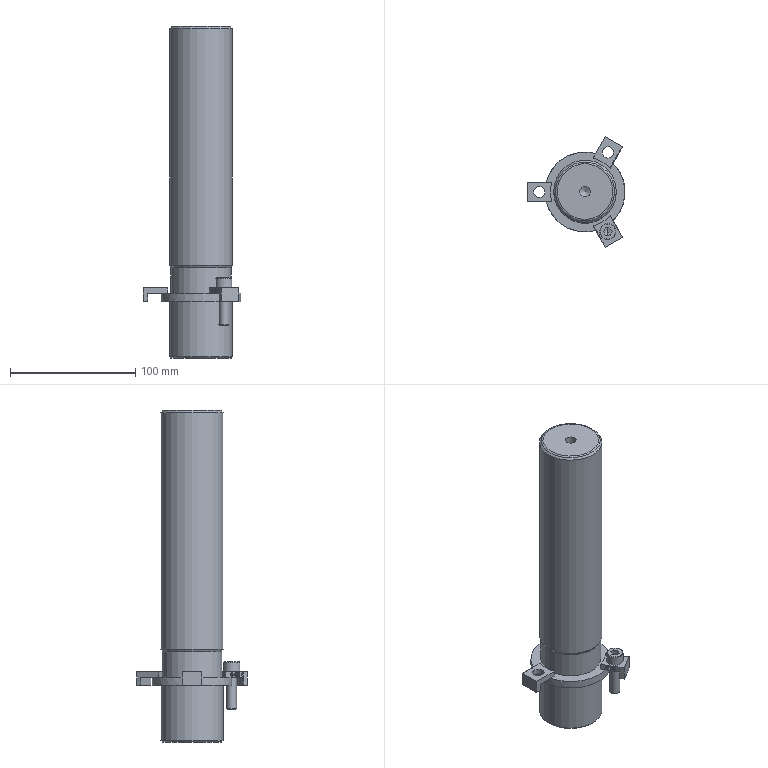Part | STEP file | lll_id3358_x_t | 1 solid | 196 faces | box 78.2 x 88.144 x 265 mm | volume 522206 mm3 | plane 118 | other 57 | cylinder 11 | cone 9 | torus 1 | commonest cylinder face diameters 9 x3 50 x2 8 x1 8.5 x1 10.5 x1 13 x1